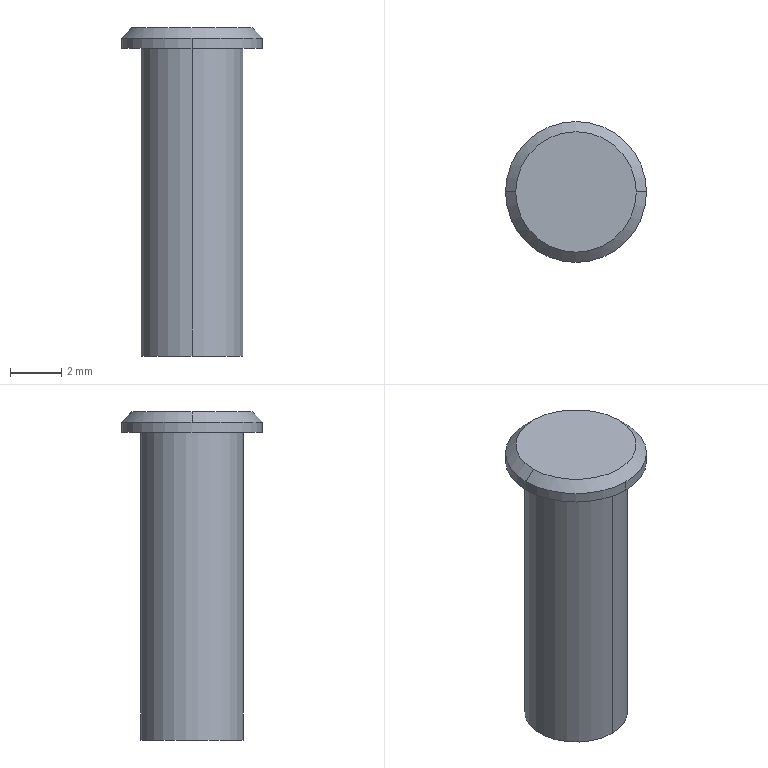Part | NX | 1 solid | 9 faces | box 5.5 x 5.5 x 12.8 mm | volume 168.488 mm3 | cylinder 4 | plane 3 | cone 2 | commonest cylinder face diameters 4 x2 5.5 x2
STEP:
#1=CARTESIAN_POINT('',(0.,-2.75,0.));
#2=VERTEX_POINT('',#1);
#3=CARTESIAN_POINT('',(0.,2.75,0.));
#4=VERTEX_POINT('',#3);
#5=CARTESIAN_POINT('',(0.,0.,0.));
#6=DIRECTION('',(0.,0.,1.));
#7=DIRECTION('',(0.,-1.,0.));
#8=AXIS2_PLACEMENT_3D('',#5,#6,#7);
#9=CIRCLE('',#8,2.75);
#10=EDGE_CURVE('',#2,#4,#9,.T.);
#11=ORIENTED_EDGE('',*,*,#10,.F.);
#12=CARTESIAN_POINT('',(0.,0.,0.));
#13=DIRECTION('',(0.,0.,1.));
#14=DIRECTION('',(0.,-1.,0.));
#15=AXIS2_PLACEMENT_3D('',#12,#13,#14);
#16=CIRCLE('',#15,2.75);
#17=EDGE_CURVE('',#4,#2,#16,.T.);
#18=ORIENTED_EDGE('',*,*,#17,.F.);
#19=EDGE_LOOP('',(#11,#18));
#20=FACE_BOUND('',#19,.T.);
#21=CARTESIAN_POINT('',(0.,2.,0.));
#22=VERTEX_POINT('',#21);
#23=CARTESIAN_POINT('',(0.,-2.,0.));
#24=VERTEX_POINT('',#23);
#25=CARTESIAN_POINT('',(0.,0.,0.));
#26=DIRECTION('',(0.,0.,-1.));
#27=DIRECTION('',(0.,1.,0.));
#28=AXIS2_PLACEMENT_3D('',#25,#26,#27);
#29=CIRCLE('',#28,2.);
#30=EDGE_CURVE('',#22,#24,#29,.T.);
#31=ORIENTED_EDGE('',*,*,#30,.F.);
#32=CARTESIAN_POINT('',(0.,0.,0.));
#33=DIRECTION('',(0.,0.,-1.));
#34=DIRECTION('',(0.,1.,0.));
#35=AXIS2_PLACEMENT_3D('',#32,#33,#34);
#36=CIRCLE('',#35,2.);
#37=EDGE_CURVE('',#24,#22,#36,.T.);
#38=ORIENTED_EDGE('',*,*,#37,.F.);
#39=EDGE_LOOP('',(#31,#38));
#40=FACE_BOUND('',#39,.T.);
#41=CARTESIAN_POINT('',(0.,0.,0.));
#42=DIRECTION('',(0.,0.,1.));
#43=DIRECTION('',(1.,0.,0.));
#44=AXIS2_PLACEMENT_3D('',#41,#42,#43);
#45=PLANE('',#44);
#46=ADVANCED_FACE('',(#20,#40),#45,.F.);
#47=ORIENTED_EDGE('',*,*,#10,.T.);
#48=CARTESIAN_POINT('',(0.,2.75,0.4));
#49=VERTEX_POINT('',#48);
#50=CARTESIAN_POINT('',(0.,2.75,0.));
#51=DIRECTION('',(0.,0.,1.));
#52=VECTOR('',#51,1000.);
#53=LINE('',#50,#52);
#54=EDGE_CURVE('',#49,#4,#53,.F.);
#55=ORIENTED_EDGE('',*,*,#54,.F.);
#56=CARTESIAN_POINT('',(2.75,0.,0.4));
#57=VERTEX_POINT('',#56);
#58=CARTESIAN_POINT('',(0.,0.,0.4));
#59=DIRECTION('',(0.,0.,-1.));
#60=DIRECTION('',(0.,-1.,0.));
#61=AXIS2_PLACEMENT_3D('',#58,#59,#60);
#62=CIRCLE('',#61,2.75);
#63=EDGE_CURVE('',#49,#57,#62,.T.);
#64=ORIENTED_EDGE('',*,*,#63,.T.);
#65=CARTESIAN_POINT('',(0.,-2.75,0.4));
#66=VERTEX_POINT('',#65);
#67=CARTESIAN_POINT('',(0.,0.,0.4));
#68=DIRECTION('',(0.,0.,-1.));
#69=DIRECTION('',(0.,-1.,0.));
#70=AXIS2_PLACEMENT_3D('',#67,#68,#69);
#71=CIRCLE('',#70,2.75);
#72=EDGE_CURVE('',#57,#66,#71,.T.);
#73=ORIENTED_EDGE('',*,*,#72,.T.);
#74=CARTESIAN_POINT('',(0.,-2.75,0.));
#75=DIRECTION('',(0.,0.,1.));
#76=VECTOR('',#75,1000.);
#77=LINE('',#74,#76);
#78=EDGE_CURVE('',#66,#2,#77,.F.);
#79=ORIENTED_EDGE('',*,*,#78,.T.);
#80=EDGE_LOOP('',(#47,#55,#64,#73,#79));
#81=FACE_BOUND('',#80,.T.);
#82=CARTESIAN_POINT('',(0.,0.,0.));
#83=DIRECTION('',(0.,0.,1.));
#84=DIRECTION('',(0.,1.,0.));
#85=AXIS2_PLACEMENT_3D('',#82,#83,#84);
#86=CYLINDRICAL_SURFACE('',#85,2.75);
#87=ADVANCED_FACE('',(#81),#86,.T.);
#88=CARTESIAN_POINT('',(0.,2.,-12.));
#89=VERTEX_POINT('',#88);
#90=CARTESIAN_POINT('',(0.,-2.,-12.));
#91=VERTEX_POINT('',#90);
#92=CARTESIAN_POINT('',(0.,0.,-12.));
#93=DIRECTION('',(0.,0.,1.));
#94=DIRECTION('',(0.,-1.,0.));
#95=AXIS2_PLACEMENT_3D('',#92,#93,#94);
#96=CIRCLE('',#95,2.);
#97=EDGE_CURVE('',#89,#91,#96,.T.);
#98=ORIENTED_EDGE('',*,*,#97,.T.);
#99=CARTESIAN_POINT('',(0.,-2.,0.));
#100=DIRECTION('',(0.,0.,-1.));
#101=VECTOR('',#100,1000.);
#102=LINE('',#99,#101);
#103=EDGE_CURVE('',#91,#24,#102,.F.);
#104=ORIENTED_EDGE('',*,*,#103,.T.);
#105=ORIENTED_EDGE('',*,*,#37,.T.);
#106=CARTESIAN_POINT('',(0.,2.,0.));
#107=DIRECTION('',(0.,0.,-1.));
#108=VECTOR('',#107,1000.);
#109=LINE('',#106,#108);
#110=EDGE_CURVE('',#89,#22,#109,.F.);
#111=ORIENTED_EDGE('',*,*,#110,.F.);
#112=EDGE_LOOP('',(#98,#104,#105,#111));
#113=FACE_BOUND('',#112,.T.);
#114=CARTESIAN_POINT('',(0.,0.,0.));
#115=DIRECTION('',(0.,0.,-1.));
#116=DIRECTION('',(0.,-1.,0.));
#117=AXIS2_PLACEMENT_3D('',#114,#115,#116);
#118=CYLINDRICAL_SURFACE('',#117,2.);
#119=ADVANCED_FACE('',(#113),#118,.T.);
#120=CARTESIAN_POINT('',(-2.35,0.,0.8));
#121=VERTEX_POINT('',#120);
#122=CARTESIAN_POINT('',(2.35,0.,0.8));
#123=VERTEX_POINT('',#122);
#124=CARTESIAN_POINT('',(0.,0.,0.8));
#125=DIRECTION('',(0.,0.,-1.));
#126=DIRECTION('',(0.,-1.,0.));
#127=AXIS2_PLACEMENT_3D('',#124,#125,#126);
#128=CIRCLE('',#127,2.35);
#129=EDGE_CURVE('',#121,#123,#128,.T.);
#130=ORIENTED_EDGE('',*,*,#129,.T.);
#131=CARTESIAN_POINT('',(2.55,0.,0.6));
#132=DIRECTION('',(0.7071,0.,-0.7071));
#133=VECTOR('',#132,1000.);
#134=LINE('',#131,#133);
#135=EDGE_CURVE('',#123,#57,#134,.T.);
#136=ORIENTED_EDGE('',*,*,#135,.T.);
#137=ORIENTED_EDGE('',*,*,#63,.F.);
#138=CARTESIAN_POINT('',(-2.75,0.,0.4));
#139=VERTEX_POINT('',#138);
#140=CARTESIAN_POINT('',(0.,0.,0.4));
#141=DIRECTION('',(0.,0.,-1.));
#142=DIRECTION('',(0.,-1.,0.));
#143=AXIS2_PLACEMENT_3D('',#140,#141,#142);
#144=CIRCLE('',#143,2.75);
#145=EDGE_CURVE('',#139,#49,#144,.T.);
#146=ORIENTED_EDGE('',*,*,#145,.F.);
#147=CARTESIAN_POINT('',(-2.55,0.,0.6));
#148=DIRECTION('',(-0.7071,0.,-0.7071));
#149=VECTOR('',#148,1000.);
#150=LINE('',#147,#149);
#151=EDGE_CURVE('',#121,#139,#150,.T.);
#152=ORIENTED_EDGE('',*,*,#151,.F.);
#153=EDGE_LOOP('',(#130,#136,#137,#146,#152));
#154=FACE_BOUND('',#153,.T.);
#155=CARTESIAN_POINT('',(0.,0.,0.6));
#156=DIRECTION('',(0.,0.,-1.));
#157=DIRECTION('',(-1.,0.,0.));
#158=AXIS2_PLACEMENT_3D('',#155,#156,#157);
#159=CONICAL_SURFACE('',#158,2.55,0.7854);
#160=ADVANCED_FACE('',(#154),#159,.T.);
#161=ORIENTED_EDGE('',*,*,#129,.F.);
#162=CARTESIAN_POINT('',(0.,0.,0.8));
#163=DIRECTION('',(0.,0.,-1.));
#164=DIRECTION('',(0.,-1.,0.));
#165=AXIS2_PLACEMENT_3D('',#162,#163,#164);
#166=CIRCLE('',#165,2.35);
#167=EDGE_CURVE('',#123,#121,#166,.T.);
#168=ORIENTED_EDGE('',*,*,#167,.F.);
#169=EDGE_LOOP('',(#161,#168));
#170=FACE_BOUND('',#169,.T.);
#171=CARTESIAN_POINT('',(0.,0.,0.8));
#172=DIRECTION('',(0.,0.,1.));
#173=DIRECTION('',(1.,0.,0.));
#174=AXIS2_PLACEMENT_3D('',#171,#172,#173);
#175=PLANE('',#174);
#176=ADVANCED_FACE('',(#170),#175,.T.);
#177=ORIENTED_EDGE('',*,*,#97,.F.);
#178=CARTESIAN_POINT('',(0.,0.,-12.));
#179=DIRECTION('',(0.,0.,1.));
#180=DIRECTION('',(0.,-1.,0.));
#181=AXIS2_PLACEMENT_3D('',#178,#179,#180);
#182=CIRCLE('',#181,2.);
#183=EDGE_CURVE('',#91,#89,#182,.T.);
#184=ORIENTED_EDGE('',*,*,#183,.F.);
#185=EDGE_LOOP('',(#177,#184));
#186=FACE_BOUND('',#185,.T.);
#187=CARTESIAN_POINT('',(0.,0.,-12.));
#188=DIRECTION('',(0.,0.,-1.));
#189=DIRECTION('',(0.,-1.,0.));
#190=AXIS2_PLACEMENT_3D('',#187,#188,#189);
#191=PLANE('',#190);
#192=ADVANCED_FACE('',(#186),#191,.T.);
#193=ORIENTED_EDGE('',*,*,#30,.T.);
#194=ORIENTED_EDGE('',*,*,#103,.F.);
#195=ORIENTED_EDGE('',*,*,#183,.T.);
#196=ORIENTED_EDGE('',*,*,#110,.T.);
#197=EDGE_LOOP('',(#193,#194,#195,#196));
#198=FACE_BOUND('',#197,.T.);
#199=CARTESIAN_POINT('',(0.,0.,0.));
#200=DIRECTION('',(0.,0.,-1.));
#201=DIRECTION('',(0.,-1.,0.));
#202=AXIS2_PLACEMENT_3D('',#199,#200,#201);
#203=CYLINDRICAL_SURFACE('',#202,2.);
#204=ADVANCED_FACE('',(#198),#203,.T.);
#205=ORIENTED_EDGE('',*,*,#72,.F.);
#206=ORIENTED_EDGE('',*,*,#135,.F.);
#207=ORIENTED_EDGE('',*,*,#167,.T.);
#208=ORIENTED_EDGE('',*,*,#151,.T.);
#209=CARTESIAN_POINT('',(0.,0.,0.4));
#210=DIRECTION('',(0.,0.,-1.));
#211=DIRECTION('',(0.,-1.,0.));
#212=AXIS2_PLACEMENT_3D('',#209,#210,#211);
#213=CIRCLE('',#212,2.75);
#214=EDGE_CURVE('',#66,#139,#213,.T.);
#215=ORIENTED_EDGE('',*,*,#214,.F.);
#216=EDGE_LOOP('',(#205,#206,#207,#208,#215));
#217=FACE_BOUND('',#216,.T.);
#218=CARTESIAN_POINT('',(0.,0.,0.6));
#219=DIRECTION('',(0.,0.,-1.));
#220=DIRECTION('',(-1.,0.,0.));
#221=AXIS2_PLACEMENT_3D('',#218,#219,#220);
#222=CONICAL_SURFACE('',#221,2.55,0.7854);
#223=ADVANCED_FACE('',(#217),#222,.T.);
#224=ORIENTED_EDGE('',*,*,#78,.F.);
#225=ORIENTED_EDGE('',*,*,#214,.T.);
#226=ORIENTED_EDGE('',*,*,#145,.T.);
#227=ORIENTED_EDGE('',*,*,#54,.T.);
#228=ORIENTED_EDGE('',*,*,#17,.T.);
#229=EDGE_LOOP('',(#224,#225,#226,#227,#228));
#230=FACE_BOUND('',#229,.T.);
#231=CARTESIAN_POINT('',(0.,0.,0.));
#232=DIRECTION('',(0.,0.,1.));
#233=DIRECTION('',(0.,1.,0.));
#234=AXIS2_PLACEMENT_3D('',#231,#232,#233);
#235=CYLINDRICAL_SURFACE('',#234,2.75);
#236=ADVANCED_FACE('',(#230),#235,.T.);
#237=CLOSED_SHELL('',(#46,#87,#119,#160,#176,#192,#204,#223,#236));
#238=MANIFOLD_SOLID_BREP('',#237);
#239=(LENGTH_UNIT()NAMED_UNIT(*)SI_UNIT(.MILLI.,.METRE.));
#240=UNCERTAINTY_MEASURE_WITH_UNIT(LENGTH_MEASURE(0.00001),#239,'','');
#241=(NAMED_UNIT(*)PLANE_ANGLE_UNIT()SI_UNIT($,.RADIAN.));
#242=(NAMED_UNIT(*)SI_UNIT($,.STERADIAN.)SOLID_ANGLE_UNIT());
#243=(GEOMETRIC_REPRESENTATION_CONTEXT(3)GLOBAL_UNCERTAINTY_ASSIGNED_CONTEXT((#240))GLOBAL_UNIT_ASSIGNED_CONTEXT((#239,#241,#242))REPRESENTATION_CONTEXT('',''));
#244=ADVANCED_BREP_SHAPE_REPRESENTATION('',(#238),#243);